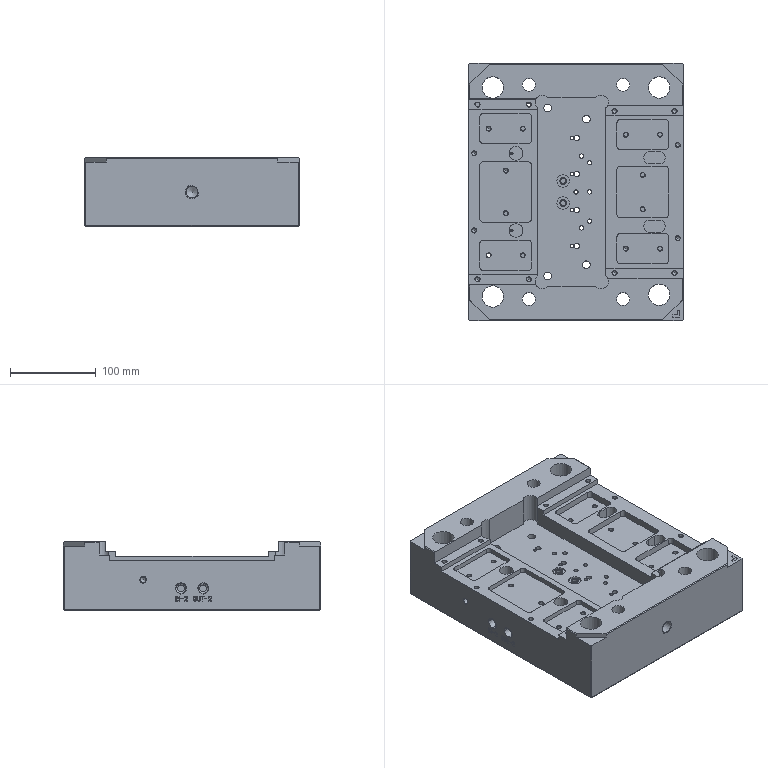NC program | PowerMill | posted with a generic post | part box 250 x 300 x 80 mm
Whole program:
%
O0001
N104 ( POWERMILL CB  : 2026004.0)
N105 ( POST VER      : 2026.0.0.5161)
N106 ( OPTION FILE   : FANUC)
N107 ( OUTPUT WORKPLANE : 1)
N108 (  )
N109 ( TOOL LIST )
N110 (-----------------------------------)
N111 ( NO. | ID    | DIA.| TIP RAD|LENGTH)
N112 (-----------------------------------)
N113 (    1|￠9_1_1| 9.0 |  0.0   |141.0 )
N114 (-----------------------------------)
N115 (  )
N116 ( NUMBER OF TOOLPATHS: 1.0 )
N117 ( ESTIMATED PROGRAM DURATION: 0 HOURS 3 MIN 55 SEC)
N118 (  )
N119 G00 G21 G80 G40 G17
N120 G90
N121 G54
N122 G53 Z0.0
N123 (---------------)
N124 ( START TOOLPATH : 03开粗-￠9-钻孔加工 )
N125 (---------------)
N126 ( TOOL NO.    :1 )
N127 ( TOOL TYPE   : DRILL)
N128 ( TOOL ID     : ￠9_1_1)
N129 ( TOOL DIA    : 9.0 LENGTH 141.0)
N130 T1
N131 M6
N132 S600 M03
N133 G00 G90 X98.0 Y33.0
N134 G43 Z20.0 H1
N135
N136 G05 P10000 R8
N137 Z11.0
N138 G01 Z-3.0 F80.0
N139 G00 Z11.0
N140 Z-2.2
N141 G01 Z-7.0
N142 G00 Z11.0
N143 Z-6.2
N144 G01 Z-11.0
N145 G00 Z11.0
N146 Z-10.2
N147 G01 Z-15.0
N148 G00 Z11.0
N149 Z-14.2
N150 G01 Z-19.0
N151 G00 Z11.0
N152 Z-18.2
N153 G01 Z-23.0
N154 G00 Z11.0
N155 Z-22.2
N156 G01 Z-27.0
N157 G00 Z11.0
N158 Z-26.2
N159 G01 Z-31.0
N160 G00 Z11.0
N161 Z-30.2
N162 G01 Z-35.0
N163 G00 Z11.0
N164 Z-34.2
N165 G01 Z-39.0
N166 G00 Z11.0
N167 Z-38.2
N168 G01 Z-43.0
N169 G00 Z11.0
N170 Z-42.2
N171 G01 Z-47.0
N172 G00 Z11.0
N173 Z-46.2
N174 G01 Z-49.7513
N175 G00 Z20.0
N176 X85.0 Y-12.0
N177 Z11.0
N178 G01 Z-3.0
N179 G00 Z11.0
N180 Z-2.2
N181 G01 Z-7.0
N182 G00 Z11.0
N183 Z-6.2
N184 G01 Z-11.0
N185 G00 Z11.0
N186 Z-10.2
N187 G01 Z-15.0
N188 G00 Z11.0
N189 Z-14.2
N190 G01 Z-19.0
N191 G00 Z11.0
N192 Z-18.2
N193 G01 Z-23.0
N194 G00 Z11.0
N195 Z-22.2
N196 G01 Z-27.0
N197 G00 Z11.0
N198 Z-26.2
N199 G01 Z-31.0
N200 G00 Z11.0
N201 Z-30.2
N202 G01 Z-35.0
N203 G00 Z11.0
N204 Z-34.2
N205 G01 Z-39.0
N206 G00 Z11.0
N207 Z-38.2
N208 G01 Z-43.0
N209 G00 Z11.0
N210 Z-42.2
N211 G01 Z-47.0
N212 G00 Z11.0
N213 Z-46.2
N214 G01 Z-49.7513
N215 G00 Z20.0
N216 X-85.0
N217 Z11.0
N218 G01 Z-3.0
N219 G00 Z11.0
N220 Z-2.2
N221 G01 Z-7.0
N222 G00 Z11.0
N223 Z-6.2
N224 G01 Z-11.0
N225 G00 Z11.0
N226 Z-10.2
N227 G01 Z-15.0
N228 G00 Z11.0
N229 Z-14.2
N230 G01 Z-19.0
N231 G00 Z11.0
N232 Z-18.2
N233 G01 Z-23.0
N234 G00 Z11.0
N235 Z-22.2
N236 G01 Z-27.0
N237 G00 Z11.0
N238 Z-26.2
N239 G01 Z-31.0
N240 G00 Z11.0
N241 Z-30.2
N242 G01 Z-35.0
N243 G00 Z11.0
N244 Z-34.2
N245 G01 Z-39.0
N246 G00 Z11.0
N247 Z-38.2
N248 G01 Z-43.0
N249 G00 Z11.0
N250 Z-42.2
N251 G01 Z-47.0
N252 G00 Z11.0
N253 Z-46.2
N254 G01 Z-49.7513
N255 G00 Z20.0
N256 X-98.0 Y33.0
N257 Z11.0
N258 G01 Z-3.0
N259 G00 Z11.0
N260 Z-2.2
N261 G01 Z-7.0
N262 G00 Z11.0
N263 Z-6.2
N264 G01 Z-11.0
N265 G00 Z11.0
N266 Z-10.2
N267 G01 Z-15.0
N268 G00 Z11.0
N269 Z-14.2
N270 G01 Z-19.0
N271 G00 Z11.0
N272 Z-18.2
N273 G01 Z-23.0
N274 G00 Z11.0
N275 Z-22.2
N276 G01 Z-27.0
N277 G00 Z11.0
N278 Z-26.2
N279 G01 Z-31.0
N280 G00 Z11.0
N281 Z-30.2
N282 G01 Z-35.0
N283 G00 Z11.0
N284 Z-34.2
N285 G01 Z-39.0
N286 G00 Z11.0
N287 Z-38.2
N288 G01 Z-43.0
N289 G00 Z11.0
N290 Z-42.2
N291 G01 Z-47.0
N292 G00 Z11.0
N293 Z-46.2
N294 G01 Z-49.7513
N295 G00 Z20.0
N296 G05 P0
N297 (---------------)
N298 ( END TOOLPATH : 03开粗-￠9-钻孔加工 )
N299 (---------------)
N300
N301 M05
N302 G53 Z0.0
N303 M30
%